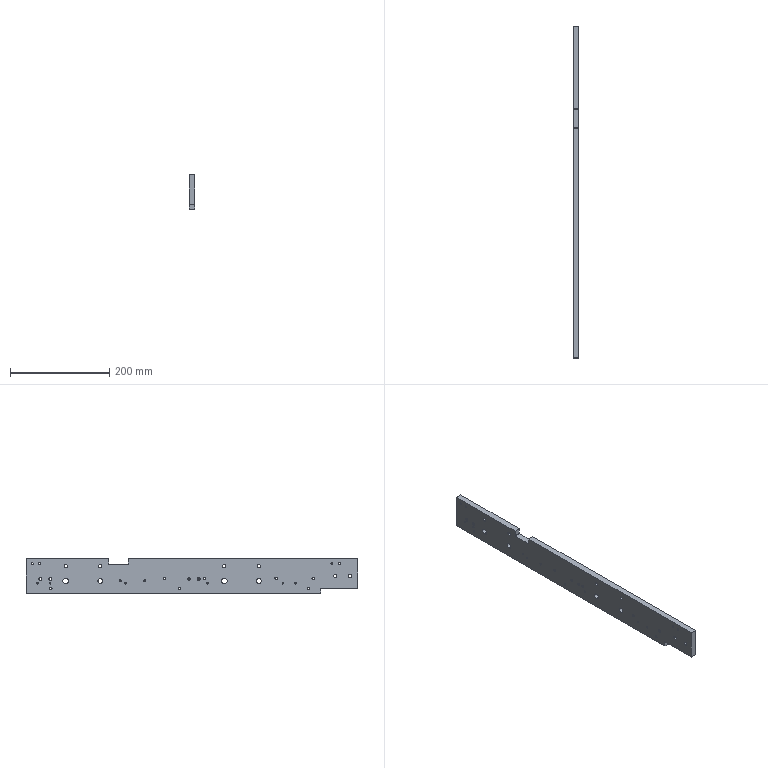Part | NX | features 5003_203_Mounting plate 2 | 1 solid | 59 faces | box 12 x 670 x 70 mm | volume 537444 mm3 | cylinder 37 | plane 16 | cone 6 | commonest cylinder face diameters 4.917 x9 4.2 x8 3.3 x6 10 x6 6.647 x4 2 x2